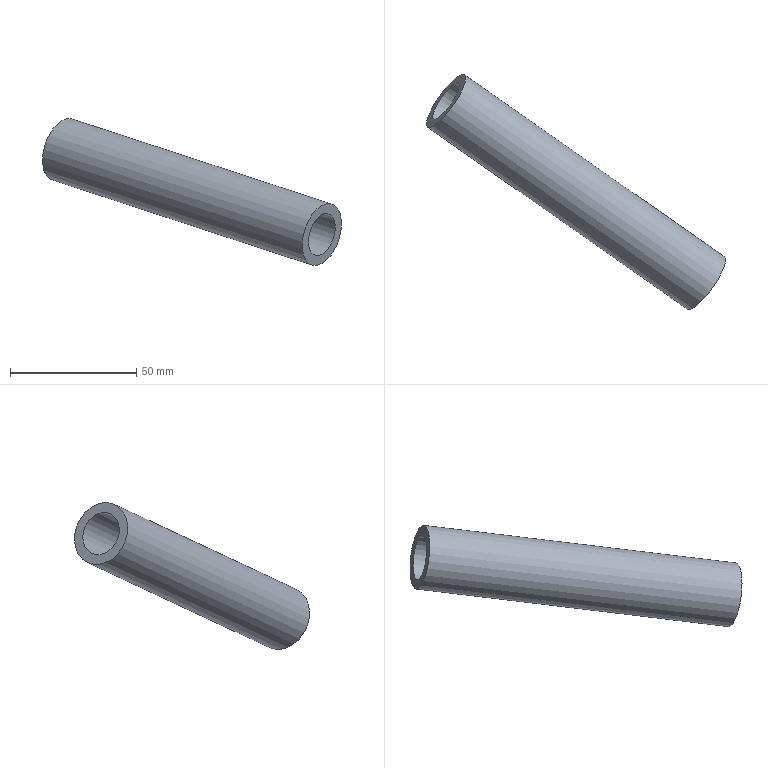Part | NX | features solid 2 | 1 solid | 4 faces | box 118.393 x 93.17 x 58.181 mm | volume 34960 mm3 | plane 2 | cylinder 2 | commonest cylinder face diameters 17.4 x1 25.4 x1
STEP:
#1=CARTESIAN_POINT('',(-803.545,437.274,-108.419));
#2=VERTEX_POINT('',#1);
#3=CARTESIAN_POINT('',(-796.26,447.678,-108.419));
#4=DIRECTION('',(-0.7912,0.554,0.2588));
#5=DIRECTION('',(-0.5736,-0.8192,0.));
#6=AXIS2_PLACEMENT_3D('',#3,#4,#5);
#7=CIRCLE('',#6,12.7);
#8=EDGE_CURVE('',#2,#2,#7,.F.);
#9=ORIENTED_EDGE('',*,*,#8,.F.);
#10=EDGE_LOOP('',(#9));
#11=FACE_BOUND('',#10,.T.);
#12=CARTESIAN_POINT('',(-801.25,440.551,-108.419));
#13=VERTEX_POINT('',#12);
#14=CARTESIAN_POINT('',(-796.26,447.678,-108.419));
#15=DIRECTION('',(-0.7912,0.554,0.2588));
#16=DIRECTION('',(-0.5736,-0.8192,0.));
#17=AXIS2_PLACEMENT_3D('',#14,#15,#16);
#18=CIRCLE('',#17,8.7);
#19=EDGE_CURVE('',#13,#13,#18,.F.);
#20=ORIENTED_EDGE('',*,*,#19,.T.);
#21=EDGE_LOOP('',(#20));
#22=FACE_BOUND('',#21,.T.);
#23=CARTESIAN_POINT('',(-796.26,447.678,-108.419));
#24=DIRECTION('',(-0.7912,0.554,0.2588));
#25=DIRECTION('',(-0.5736,-0.8192,0.));
#26=AXIS2_PLACEMENT_3D('',#23,#24,#25);
#27=PLANE('',#26);
#28=ADVANCED_FACE('',(#11,#22),#27,.T.);
#29=CARTESIAN_POINT('',(-700.683,365.25,-142.065));
#30=VERTEX_POINT('',#29);
#31=CARTESIAN_POINT('',(-693.399,375.653,-142.065));
#32=DIRECTION('',(-0.7912,0.554,0.2588));
#33=DIRECTION('',(-0.5736,-0.8192,0.));
#34=AXIS2_PLACEMENT_3D('',#31,#32,#33);
#35=CIRCLE('',#34,12.7);
#36=EDGE_CURVE('',#30,#30,#35,.F.);
#37=ORIENTED_EDGE('',*,*,#36,.T.);
#38=EDGE_LOOP('',(#37));
#39=FACE_BOUND('',#38,.T.);
#40=CARTESIAN_POINT('',(-688.409,382.78,-142.065));
#41=VERTEX_POINT('',#40);
#42=CARTESIAN_POINT('',(-693.399,375.653,-142.065));
#43=DIRECTION('',(0.7912,-0.554,-0.2588));
#44=DIRECTION('',(0.5736,0.8192,0.));
#45=AXIS2_PLACEMENT_3D('',#42,#43,#44);
#46=CIRCLE('',#45,8.7);
#47=EDGE_CURVE('',#41,#41,#46,.T.);
#48=ORIENTED_EDGE('',*,*,#47,.F.);
#49=EDGE_LOOP('',(#48));
#50=FACE_BOUND('',#49,.T.);
#51=CARTESIAN_POINT('',(-693.399,375.653,-142.065));
#52=DIRECTION('',(-0.7912,0.554,0.2588));
#53=DIRECTION('',(-0.5736,-0.8192,0.));
#54=AXIS2_PLACEMENT_3D('',#51,#52,#53);
#55=PLANE('',#54);
#56=ADVANCED_FACE('',(#39,#50),#55,.F.);
#57=ORIENTED_EDGE('',*,*,#8,.T.);
#58=EDGE_LOOP('',(#57));
#59=FACE_BOUND('',#58,.T.);
#60=ORIENTED_EDGE('',*,*,#36,.F.);
#61=EDGE_LOOP('',(#60));
#62=FACE_BOUND('',#61,.T.);
#63=CARTESIAN_POINT('',(-693.399,375.653,-142.065));
#64=DIRECTION('',(-0.7912,0.554,0.2588));
#65=DIRECTION('',(-0.5736,-0.8192,0.));
#66=AXIS2_PLACEMENT_3D('',#63,#64,#65);
#67=CYLINDRICAL_SURFACE('',#66,12.7);
#68=ADVANCED_FACE('',(#59,#62),#67,.T.);
#69=ORIENTED_EDGE('',*,*,#19,.F.);
#70=EDGE_LOOP('',(#69));
#71=FACE_BOUND('',#70,.T.);
#72=ORIENTED_EDGE('',*,*,#47,.T.);
#73=EDGE_LOOP('',(#72));
#74=FACE_BOUND('',#73,.T.);
#75=CARTESIAN_POINT('',(-693.399,375.653,-142.065));
#76=DIRECTION('',(-0.7912,0.554,0.2588));
#77=DIRECTION('',(-0.5736,-0.8192,0.));
#78=AXIS2_PLACEMENT_3D('',#75,#76,#77);
#79=CYLINDRICAL_SURFACE('',#78,8.7);
#80=ADVANCED_FACE('',(#71,#74),#79,.F.);
#81=CLOSED_SHELL('',(#28,#56,#68,#80));
#82=MANIFOLD_SOLID_BREP('',#81);
#83=(LENGTH_UNIT()NAMED_UNIT(*)SI_UNIT(.MILLI.,.METRE.));
#84=UNCERTAINTY_MEASURE_WITH_UNIT(LENGTH_MEASURE(0.00001),#83,'','');
#85=(NAMED_UNIT(*)PLANE_ANGLE_UNIT()SI_UNIT($,.RADIAN.));
#86=(NAMED_UNIT(*)SI_UNIT($,.STERADIAN.)SOLID_ANGLE_UNIT());
#87=(GEOMETRIC_REPRESENTATION_CONTEXT(3)GLOBAL_UNCERTAINTY_ASSIGNED_CONTEXT((#84))GLOBAL_UNIT_ASSIGNED_CONTEXT((#83,#85,#86))REPRESENTATION_CONTEXT('',''));
#88=ADVANCED_BREP_SHAPE_REPRESENTATION('',(#82),#87);